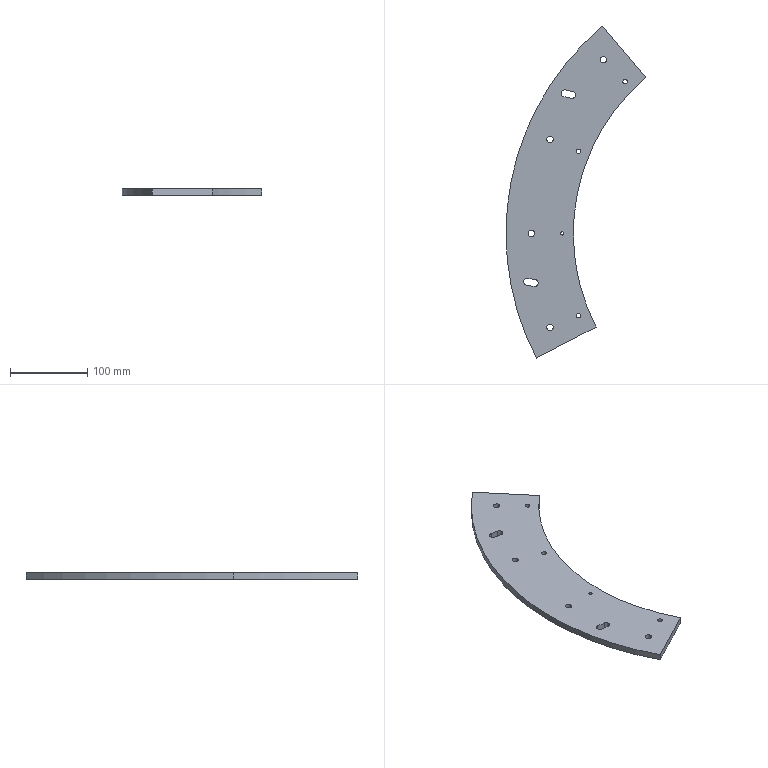Part | 1 solid | 33 faces | box 180.849 x 428.908 x 8 mm | volume 283021 mm3 | cylinder 25 | plane 8 | commonest cylinder face diameters 8.2 x8 6 x6 9 x6 4.174 x2 700 x2 526 x1
STEP:
#1=CARTESIAN_POINT('',(-308.372,-64.185,0.));
#2=VERTEX_POINT('',#1);
#3=CARTESIAN_POINT('',(-311.994,-59.771,0.));
#4=VERTEX_POINT('',#3);
#5=CARTESIAN_POINT('',(-312.872,-64.185,0.));
#6=DIRECTION('',(0.,0.,1.));
#7=DIRECTION('',(1.,0.,0.));
#8=AXIS2_PLACEMENT_3D('',#5,#6,#7);
#9=CIRCLE('',#8,4.5);
#10=EDGE_CURVE('',#2,#4,#9,.T.);
#11=ORIENTED_EDGE('',*,*,#10,.F.);
#12=CARTESIAN_POINT('',(-308.372,-64.185,8.));
#13=VERTEX_POINT('',#12);
#14=CARTESIAN_POINT('',(-308.372,-64.185,-2.));
#15=DIRECTION('',(0.,0.,1.));
#16=VECTOR('',#15,1000.);
#17=LINE('',#14,#16);
#18=EDGE_CURVE('',#2,#13,#17,.T.);
#19=ORIENTED_EDGE('',*,*,#18,.T.);
#20=CARTESIAN_POINT('',(-311.994,-59.771,8.));
#21=VERTEX_POINT('',#20);
#22=CARTESIAN_POINT('',(-312.872,-64.185,8.));
#23=DIRECTION('',(0.,0.,1.));
#24=DIRECTION('',(1.,0.,0.));
#25=AXIS2_PLACEMENT_3D('',#22,#23,#24);
#26=CIRCLE('',#25,4.5);
#27=EDGE_CURVE('',#13,#21,#26,.T.);
#28=ORIENTED_EDGE('',*,*,#27,.T.);
#29=CARTESIAN_POINT('',(-311.994,-59.771,-2.));
#30=DIRECTION('',(0.,0.,1.));
#31=VECTOR('',#30,1000.);
#32=LINE('',#29,#31);
#33=EDGE_CURVE('',#4,#21,#32,.T.);
#34=ORIENTED_EDGE('',*,*,#33,.F.);
#35=EDGE_LOOP('',(#11,#19,#28,#34));
#36=FACE_OUTER_BOUND('',#35,.T.);
#37=CARTESIAN_POINT('',(-312.872,-64.185,-2.));
#38=DIRECTION('',(0.,0.,1.));
#39=DIRECTION('',(1.,0.,0.));
#40=AXIS2_PLACEMENT_3D('',#37,#38,#39);
#41=CYLINDRICAL_SURFACE('',#40,4.5);
#42=ADVANCED_FACE('',(#36),#41,.F.);
#43=CARTESIAN_POINT('',(-259.993,179.03,0.));
#44=VERTEX_POINT('',#43);
#45=CARTESIAN_POINT('',(-263.616,183.444,0.));
#46=VERTEX_POINT('',#45);
#47=CARTESIAN_POINT('',(-264.493,179.03,0.));
#48=DIRECTION('',(0.,0.,1.));
#49=DIRECTION('',(1.,0.,0.));
#50=AXIS2_PLACEMENT_3D('',#47,#48,#49);
#51=CIRCLE('',#50,4.5);
#52=EDGE_CURVE('',#44,#46,#51,.T.);
#53=ORIENTED_EDGE('',*,*,#52,.F.);
#54=CARTESIAN_POINT('',(-259.993,179.03,8.));
#55=VERTEX_POINT('',#54);
#56=CARTESIAN_POINT('',(-259.993,179.03,-2.));
#57=DIRECTION('',(0.,0.,1.));
#58=VECTOR('',#57,1000.);
#59=LINE('',#56,#58);
#60=EDGE_CURVE('',#44,#55,#59,.T.);
#61=ORIENTED_EDGE('',*,*,#60,.T.);
#62=CARTESIAN_POINT('',(-263.616,183.444,8.));
#63=VERTEX_POINT('',#62);
#64=CARTESIAN_POINT('',(-264.493,179.03,8.));
#65=DIRECTION('',(0.,0.,1.));
#66=DIRECTION('',(1.,0.,0.));
#67=AXIS2_PLACEMENT_3D('',#64,#65,#66);
#68=CIRCLE('',#67,4.5);
#69=EDGE_CURVE('',#55,#63,#68,.T.);
#70=ORIENTED_EDGE('',*,*,#69,.T.);
#71=CARTESIAN_POINT('',(-263.616,183.444,-2.));
#72=DIRECTION('',(0.,0.,1.));
#73=VECTOR('',#72,1000.);
#74=LINE('',#71,#73);
#75=EDGE_CURVE('',#46,#63,#74,.T.);
#76=ORIENTED_EDGE('',*,*,#75,.F.);
#77=EDGE_LOOP('',(#53,#61,#70,#76));
#78=FACE_OUTER_BOUND('',#77,.T.);
#79=CARTESIAN_POINT('',(-264.493,179.03,-2.));
#80=DIRECTION('',(0.,0.,1.));
#81=DIRECTION('',(1.,0.,0.));
#82=AXIS2_PLACEMENT_3D('',#79,#80,#81);
#83=CYLINDRICAL_SURFACE('',#82,4.5);
#84=ADVANCED_FACE('',(#78),#83,.F.);
#85=CARTESIAN_POINT('',(-228.457,224.357,0.));
#86=VERTEX_POINT('',#85);
#87=CARTESIAN_POINT('',(-220.257,224.357,0.));
#88=VERTEX_POINT('',#87);
#89=CARTESIAN_POINT('',(-224.357,224.357,0.));
#90=DIRECTION('',(0.,0.,1.));
#91=DIRECTION('',(1.,0.,0.));
#92=AXIS2_PLACEMENT_3D('',#89,#90,#91);
#93=CIRCLE('',#92,4.1);
#94=EDGE_CURVE('',#86,#88,#93,.T.);
#95=ORIENTED_EDGE('',*,*,#94,.F.);
#96=CARTESIAN_POINT('',(-228.457,224.357,8.));
#97=VERTEX_POINT('',#96);
#98=CARTESIAN_POINT('',(-228.457,224.357,-2.));
#99=DIRECTION('',(0.,0.,1.));
#100=VECTOR('',#99,1000.);
#101=LINE('',#98,#100);
#102=EDGE_CURVE('',#86,#97,#101,.T.);
#103=ORIENTED_EDGE('',*,*,#102,.T.);
#104=CARTESIAN_POINT('',(-220.257,224.357,8.));
#105=VERTEX_POINT('',#104);
#106=CARTESIAN_POINT('',(-224.357,224.357,8.));
#107=DIRECTION('',(0.,0.,1.));
#108=DIRECTION('',(1.,0.,0.));
#109=AXIS2_PLACEMENT_3D('',#106,#107,#108);
#110=CIRCLE('',#109,4.1);
#111=EDGE_CURVE('',#97,#105,#110,.T.);
#112=ORIENTED_EDGE('',*,*,#111,.T.);
#113=CARTESIAN_POINT('',(-220.257,224.357,-2.));
#114=DIRECTION('',(0.,0.,1.));
#115=VECTOR('',#114,1000.);
#116=LINE('',#113,#115);
#117=EDGE_CURVE('',#88,#105,#116,.T.);
#118=ORIENTED_EDGE('',*,*,#117,.F.);
#119=EDGE_LOOP('',(#95,#103,#112,#118));
#120=FACE_OUTER_BOUND('',#119,.T.);
#121=CARTESIAN_POINT('',(-224.357,224.357,-2.));
#122=DIRECTION('',(0.,0.,1.));
#123=DIRECTION('',(1.,0.,0.));
#124=AXIS2_PLACEMENT_3D('',#121,#122,#123);
#125=CYLINDRICAL_SURFACE('',#124,4.1);
#126=ADVANCED_FACE('',(#120),#125,.F.);
#127=CARTESIAN_POINT('',(-297.237,121.421,0.));
#128=VERTEX_POINT('',#127);
#129=CARTESIAN_POINT('',(-289.037,121.421,0.));
#130=VERTEX_POINT('',#129);
#131=CARTESIAN_POINT('',(-293.137,121.421,0.));
#132=DIRECTION('',(0.,0.,1.));
#133=DIRECTION('',(1.,0.,0.));
#134=AXIS2_PLACEMENT_3D('',#131,#132,#133);
#135=CIRCLE('',#134,4.1);
#136=EDGE_CURVE('',#128,#130,#135,.T.);
#137=ORIENTED_EDGE('',*,*,#136,.F.);
#138=CARTESIAN_POINT('',(-297.237,121.421,8.));
#139=VERTEX_POINT('',#138);
#140=CARTESIAN_POINT('',(-297.237,121.421,-2.));
#141=DIRECTION('',(0.,0.,1.));
#142=VECTOR('',#141,1000.);
#143=LINE('',#140,#142);
#144=EDGE_CURVE('',#128,#139,#143,.T.);
#145=ORIENTED_EDGE('',*,*,#144,.T.);
#146=CARTESIAN_POINT('',(-289.037,121.421,8.));
#147=VERTEX_POINT('',#146);
#148=CARTESIAN_POINT('',(-293.137,121.421,8.));
#149=DIRECTION('',(0.,0.,1.));
#150=DIRECTION('',(1.,0.,0.));
#151=AXIS2_PLACEMENT_3D('',#148,#149,#150);
#152=CIRCLE('',#151,4.1);
#153=EDGE_CURVE('',#139,#147,#152,.T.);
#154=ORIENTED_EDGE('',*,*,#153,.T.);
#155=CARTESIAN_POINT('',(-289.037,121.421,-2.));
#156=DIRECTION('',(0.,0.,1.));
#157=VECTOR('',#156,1000.);
#158=LINE('',#155,#157);
#159=EDGE_CURVE('',#130,#147,#158,.T.);
#160=ORIENTED_EDGE('',*,*,#159,.F.);
#161=EDGE_LOOP('',(#137,#145,#154,#160));
#162=FACE_OUTER_BOUND('',#161,.T.);
#163=CARTESIAN_POINT('',(-293.137,121.421,-2.));
#164=DIRECTION('',(0.,0.,1.));
#165=DIRECTION('',(1.,0.,0.));
#166=AXIS2_PLACEMENT_3D('',#163,#164,#165);
#167=CYLINDRICAL_SURFACE('',#166,4.1);
#168=ADVANCED_FACE('',(#162),#167,.F.);
#169=CARTESIAN_POINT('',(-321.389,0.,0.));
#170=VERTEX_POINT('',#169);
#171=CARTESIAN_POINT('',(-313.189,0.,0.));
#172=VERTEX_POINT('',#171);
#173=CARTESIAN_POINT('',(-317.289,0.,0.));
#174=DIRECTION('',(0.,0.,1.));
#175=DIRECTION('',(1.,0.,0.));
#176=AXIS2_PLACEMENT_3D('',#173,#174,#175);
#177=CIRCLE('',#176,4.1);
#178=EDGE_CURVE('',#170,#172,#177,.T.);
#179=ORIENTED_EDGE('',*,*,#178,.F.);
#180=CARTESIAN_POINT('',(-321.389,0.,8.));
#181=VERTEX_POINT('',#180);
#182=CARTESIAN_POINT('',(-321.389,0.,-2.));
#183=DIRECTION('',(0.,0.,1.));
#184=VECTOR('',#183,1000.);
#185=LINE('',#182,#184);
#186=EDGE_CURVE('',#170,#181,#185,.T.);
#187=ORIENTED_EDGE('',*,*,#186,.T.);
#188=CARTESIAN_POINT('',(-313.189,0.,8.));
#189=VERTEX_POINT('',#188);
#190=CARTESIAN_POINT('',(-317.289,0.,8.));
#191=DIRECTION('',(0.,0.,1.));
#192=DIRECTION('',(1.,0.,0.));
#193=AXIS2_PLACEMENT_3D('',#190,#191,#192);
#194=CIRCLE('',#193,4.1);
#195=EDGE_CURVE('',#181,#189,#194,.T.);
#196=ORIENTED_EDGE('',*,*,#195,.T.);
#197=CARTESIAN_POINT('',(-313.189,0.,-2.));
#198=DIRECTION('',(0.,0.,1.));
#199=VECTOR('',#198,1000.);
#200=LINE('',#197,#199);
#201=EDGE_CURVE('',#172,#189,#200,.T.);
#202=ORIENTED_EDGE('',*,*,#201,.F.);
#203=EDGE_LOOP('',(#179,#187,#196,#202));
#204=FACE_OUTER_BOUND('',#203,.T.);
#205=CARTESIAN_POINT('',(-317.289,0.,-2.));
#206=DIRECTION('',(0.,0.,1.));
#207=DIRECTION('',(1.,0.,0.));
#208=AXIS2_PLACEMENT_3D('',#205,#206,#207);
#209=CYLINDRICAL_SURFACE('',#208,4.1);
#210=ADVANCED_FACE('',(#204),#209,.F.);
#211=CARTESIAN_POINT('',(-297.237,-121.421,0.));
#212=VERTEX_POINT('',#211);
#213=CARTESIAN_POINT('',(-289.037,-121.421,0.));
#214=VERTEX_POINT('',#213);
#215=CARTESIAN_POINT('',(-293.137,-121.421,0.));
#216=DIRECTION('',(0.,0.,1.));
#217=DIRECTION('',(1.,0.,0.));
#218=AXIS2_PLACEMENT_3D('',#215,#216,#217);
#219=CIRCLE('',#218,4.1);
#220=EDGE_CURVE('',#212,#214,#219,.T.);
#221=ORIENTED_EDGE('',*,*,#220,.F.);
#222=CARTESIAN_POINT('',(-297.237,-121.421,8.));
#223=VERTEX_POINT('',#222);
#224=CARTESIAN_POINT('',(-297.237,-121.421,-2.));
#225=DIRECTION('',(0.,0.,1.));
#226=VECTOR('',#225,1000.);
#227=LINE('',#224,#226);
#228=EDGE_CURVE('',#212,#223,#227,.T.);
#229=ORIENTED_EDGE('',*,*,#228,.T.);
#230=CARTESIAN_POINT('',(-289.037,-121.421,8.));
#231=VERTEX_POINT('',#230);
#232=CARTESIAN_POINT('',(-293.137,-121.421,8.));
#233=DIRECTION('',(0.,0.,1.));
#234=DIRECTION('',(1.,0.,0.));
#235=AXIS2_PLACEMENT_3D('',#232,#233,#234);
#236=CIRCLE('',#235,4.1);
#237=EDGE_CURVE('',#223,#231,#236,.T.);
#238=ORIENTED_EDGE('',*,*,#237,.T.);
#239=CARTESIAN_POINT('',(-289.037,-121.421,-2.));
#240=DIRECTION('',(0.,0.,1.));
#241=VECTOR('',#240,1000.);
#242=LINE('',#239,#241);
#243=EDGE_CURVE('',#214,#231,#242,.T.);
#244=ORIENTED_EDGE('',*,*,#243,.F.);
#245=EDGE_LOOP('',(#221,#229,#238,#244));
#246=FACE_OUTER_BOUND('',#245,.T.);
#247=CARTESIAN_POINT('',(-293.137,-121.421,-2.));
#248=DIRECTION('',(0.,0.,1.));
#249=DIRECTION('',(1.,0.,0.));
#250=AXIS2_PLACEMENT_3D('',#247,#248,#249);
#251=CYLINDRICAL_SURFACE('',#250,4.1);
#252=ADVANCED_FACE('',(#246),#251,.F.);
#253=CARTESIAN_POINT('',(-259.182,-106.114,0.));
#254=VERTEX_POINT('',#253);
#255=CARTESIAN_POINT('',(-253.182,-106.114,0.));
#256=VERTEX_POINT('',#255);
#257=CARTESIAN_POINT('',(-256.182,-106.114,0.));
#258=DIRECTION('',(0.,0.,1.));
#259=DIRECTION('',(1.,0.,0.));
#260=AXIS2_PLACEMENT_3D('',#257,#258,#259);
#261=CIRCLE('',#260,3.);
#262=EDGE_CURVE('',#254,#256,#261,.T.);
#263=ORIENTED_EDGE('',*,*,#262,.F.);
#264=CARTESIAN_POINT('',(-259.182,-106.114,8.));
#265=VERTEX_POINT('',#264);
#266=CARTESIAN_POINT('',(-259.182,-106.114,0.));
#267=DIRECTION('',(0.,0.,1.));
#268=VECTOR('',#267,1000.);
#269=LINE('',#266,#268);
#270=EDGE_CURVE('',#254,#265,#269,.T.);
#271=ORIENTED_EDGE('',*,*,#270,.T.);
#272=CARTESIAN_POINT('',(-253.182,-106.114,8.));
#273=VERTEX_POINT('',#272);
#274=CARTESIAN_POINT('',(-256.182,-106.114,8.));
#275=DIRECTION('',(0.,0.,1.));
#276=DIRECTION('',(1.,0.,0.));
#277=AXIS2_PLACEMENT_3D('',#274,#275,#276);
#278=CIRCLE('',#277,3.);
#279=EDGE_CURVE('',#265,#273,#278,.T.);
#280=ORIENTED_EDGE('',*,*,#279,.T.);
#281=CARTESIAN_POINT('',(-253.182,-106.114,0.));
#282=DIRECTION('',(0.,0.,1.));
#283=VECTOR('',#282,1000.);
#284=LINE('',#281,#283);
#285=EDGE_CURVE('',#256,#273,#284,.T.);
#286=ORIENTED_EDGE('',*,*,#285,.F.);
#287=EDGE_LOOP('',(#263,#271,#280,#286));
#288=FACE_OUTER_BOUND('',#287,.T.);
#289=CARTESIAN_POINT('',(-256.182,-106.114,0.));
#290=DIRECTION('',(0.,0.,1.));
#291=DIRECTION('',(1.,0.,0.));
#292=AXIS2_PLACEMENT_3D('',#289,#290,#291);
#293=CYLINDRICAL_SURFACE('',#292,3.);
#294=ADVANCED_FACE('',(#288),#293,.F.);
#295=CARTESIAN_POINT('',(-279.376,0.,0.));
#296=VERTEX_POINT('',#295);
#297=CARTESIAN_POINT('',(-275.202,0.,0.));
#298=VERTEX_POINT('',#297);
#299=CARTESIAN_POINT('',(-277.289,0.,0.));
#300=DIRECTION('',(0.,0.,1.));
#301=DIRECTION('',(1.,0.,0.));
#302=AXIS2_PLACEMENT_3D('',#299,#300,#301);
#303=CIRCLE('',#302,2.087);
#304=EDGE_CURVE('',#296,#298,#303,.T.);
#305=ORIENTED_EDGE('',*,*,#304,.F.);
#306=CARTESIAN_POINT('',(-279.376,0.,8.));
#307=VERTEX_POINT('',#306);
#308=CARTESIAN_POINT('',(-279.376,0.,0.));
#309=DIRECTION('',(0.,0.,1.));
#310=VECTOR('',#309,1000.);
#311=LINE('',#308,#310);
#312=EDGE_CURVE('',#296,#307,#311,.T.);
#313=ORIENTED_EDGE('',*,*,#312,.T.);
#314=CARTESIAN_POINT('',(-275.202,0.,8.));
#315=VERTEX_POINT('',#314);
#316=CARTESIAN_POINT('',(-277.289,0.,8.));
#317=DIRECTION('',(0.,0.,1.));
#318=DIRECTION('',(1.,0.,0.));
#319=AXIS2_PLACEMENT_3D('',#316,#317,#318);
#320=CIRCLE('',#319,2.087);
#321=EDGE_CURVE('',#307,#315,#320,.T.);
#322=ORIENTED_EDGE('',*,*,#321,.T.);
#323=CARTESIAN_POINT('',(-275.202,0.,0.));
#324=DIRECTION('',(0.,0.,1.));
#325=VECTOR('',#324,1000.);
#326=LINE('',#323,#325);
#327=EDGE_CURVE('',#298,#315,#326,.T.);
#328=ORIENTED_EDGE('',*,*,#327,.F.);
#329=EDGE_LOOP('',(#305,#313,#322,#328));
#330=FACE_OUTER_BOUND('',#329,.T.);
#331=CARTESIAN_POINT('',(-277.289,0.,0.));
#332=DIRECTION('',(0.,0.,1.));
#333=DIRECTION('',(1.,0.,0.));
#334=AXIS2_PLACEMENT_3D('',#331,#332,#333);
#335=CYLINDRICAL_SURFACE('',#334,2.087);
#336=ADVANCED_FACE('',(#330),#335,.F.);
#337=CARTESIAN_POINT('',(-259.182,106.114,0.));
#338=VERTEX_POINT('',#337);
#339=CARTESIAN_POINT('',(-253.182,106.114,0.));
#340=VERTEX_POINT('',#339);
#341=CARTESIAN_POINT('',(-256.182,106.114,0.));
#342=DIRECTION('',(0.,0.,1.));
#343=DIRECTION('',(1.,0.,0.));
#344=AXIS2_PLACEMENT_3D('',#341,#342,#343);
#345=CIRCLE('',#344,3.);
#346=EDGE_CURVE('',#338,#340,#345,.T.);
#347=ORIENTED_EDGE('',*,*,#346,.F.);
#348=CARTESIAN_POINT('',(-259.182,106.114,8.));
#349=VERTEX_POINT('',#348);
#350=CARTESIAN_POINT('',(-259.182,106.114,0.));
#351=DIRECTION('',(0.,0.,1.));
#352=VECTOR('',#351,1000.);
#353=LINE('',#350,#352);
#354=EDGE_CURVE('',#338,#349,#353,.T.);
#355=ORIENTED_EDGE('',*,*,#354,.T.);
#356=CARTESIAN_POINT('',(-253.182,106.114,8.));
#357=VERTEX_POINT('',#356);
#358=CARTESIAN_POINT('',(-256.182,106.114,8.));
#359=DIRECTION('',(0.,0.,1.));
#360=DIRECTION('',(1.,0.,0.));
#361=AXIS2_PLACEMENT_3D('',#358,#359,#360);
#362=CIRCLE('',#361,3.);
#363=EDGE_CURVE('',#349,#357,#362,.T.);
#364=ORIENTED_EDGE('',*,*,#363,.T.);
#365=CARTESIAN_POINT('',(-253.182,106.114,0.));
#366=DIRECTION('',(0.,0.,1.));
#367=VECTOR('',#366,1000.);
#368=LINE('',#365,#367);
#369=EDGE_CURVE('',#340,#357,#368,.T.);
#370=ORIENTED_EDGE('',*,*,#369,.F.);
#371=EDGE_LOOP('',(#347,#355,#364,#370));
#372=FACE_OUTER_BOUND('',#371,.T.);
#373=CARTESIAN_POINT('',(-256.182,106.114,0.));
#374=DIRECTION('',(0.,0.,1.));
#375=DIRECTION('',(1.,0.,0.));
#376=AXIS2_PLACEMENT_3D('',#373,#374,#375);
#377=CYLINDRICAL_SURFACE('',#376,3.);
#378=ADVANCED_FACE('',(#372),#377,.F.);
#379=CARTESIAN_POINT('',(-199.073,196.073,0.));
#380=VERTEX_POINT('',#379);
#381=CARTESIAN_POINT('',(-193.073,196.073,0.));
#382=VERTEX_POINT('',#381);
#383=CARTESIAN_POINT('',(-196.073,196.073,0.));
#384=DIRECTION('',(0.,0.,1.));
#385=DIRECTION('',(1.,0.,0.));
#386=AXIS2_PLACEMENT_3D('',#383,#384,#385);
#387=CIRCLE('',#386,3.);
#388=EDGE_CURVE('',#380,#382,#387,.T.);
#389=ORIENTED_EDGE('',*,*,#388,.F.);
#390=CARTESIAN_POINT('',(-199.073,196.073,8.));
#391=VERTEX_POINT('',#390);
#392=CARTESIAN_POINT('',(-199.073,196.073,0.));
#393=DIRECTION('',(0.,0.,1.));
#394=VECTOR('',#393,1000.);
#395=LINE('',#392,#394);
#396=EDGE_CURVE('',#380,#391,#395,.T.);
#397=ORIENTED_EDGE('',*,*,#396,.T.);
#398=CARTESIAN_POINT('',(-193.073,196.073,8.));
#399=VERTEX_POINT('',#398);
#400=CARTESIAN_POINT('',(-196.073,196.073,8.));
#401=DIRECTION('',(0.,0.,1.));
#402=DIRECTION('',(1.,0.,0.));
#403=AXIS2_PLACEMENT_3D('',#400,#401,#402);
#404=CIRCLE('',#403,3.);
#405=EDGE_CURVE('',#391,#399,#404,.T.);
#406=ORIENTED_EDGE('',*,*,#405,.T.);
#407=CARTESIAN_POINT('',(-193.073,196.073,0.));
#408=DIRECTION('',(0.,0.,1.));
#409=VECTOR('',#408,1000.);
#410=LINE('',#407,#409);
#411=EDGE_CURVE('',#382,#399,#410,.T.);
#412=ORIENTED_EDGE('',*,*,#411,.F.);
#413=EDGE_LOOP('',(#389,#397,#406,#412));
#414=FACE_OUTER_BOUND('',#413,.T.);
#415=CARTESIAN_POINT('',(-196.073,196.073,0.));
#416=DIRECTION('',(0.,0.,1.));
#417=DIRECTION('',(1.,0.,0.));
#418=AXIS2_PLACEMENT_3D('',#415,#416,#417);
#419=CYLINDRICAL_SURFACE('',#418,3.);
#420=ADVANCED_FACE('',(#414),#419,.F.);
#421=CARTESIAN_POINT('',(-350.,0.,8.));
#422=VERTEX_POINT('',#421);
#423=CARTESIAN_POINT('',(-310.823,-160.901,8.));
#424=VERTEX_POINT('',#423);
#425=CARTESIAN_POINT('',(0.,0.,8.));
#426=DIRECTION('',(0.,0.,1.));
#427=DIRECTION('',(1.,0.,0.));
#428=AXIS2_PLACEMENT_3D('',#425,#426,#427);
#429=CIRCLE('',#428,350.);
#430=EDGE_CURVE('',#422,#424,#429,.T.);
#431=ORIENTED_EDGE('',*,*,#430,.F.);
#432=CARTESIAN_POINT('',(-350.,0.,0.));
#433=VERTEX_POINT('',#432);
#434=CARTESIAN_POINT('',(-350.,0.,8.));
#435=DIRECTION('',(0.,0.,-1.));
#436=VECTOR('',#435,1000.);
#437=LINE('',#434,#436);
#438=EDGE_CURVE('',#422,#433,#437,.T.);
#439=ORIENTED_EDGE('',*,*,#438,.T.);
#440=CARTESIAN_POINT('',(-310.823,-160.901,0.));
#441=VERTEX_POINT('',#440);
#442=CARTESIAN_POINT('',(0.,0.,0.));
#443=DIRECTION('',(0.,0.,1.));
#444=DIRECTION('',(1.,0.,0.));
#445=AXIS2_PLACEMENT_3D('',#442,#443,#444);
#446=CIRCLE('',#445,350.);
#447=EDGE_CURVE('',#433,#441,#446,.T.);
#448=ORIENTED_EDGE('',*,*,#447,.T.);
#449=CARTESIAN_POINT('',(-310.823,-160.901,-44.));
#450=DIRECTION('',(0.,0.,1.));
#451=VECTOR('',#450,1000.);
#452=LINE('',#449,#451);
#453=EDGE_CURVE('',#441,#424,#452,.T.);
#454=ORIENTED_EDGE('',*,*,#453,.T.);
#455=EDGE_LOOP('',(#431,#439,#448,#454));
#456=FACE_OUTER_BOUND('',#455,.T.);
#457=CARTESIAN_POINT('',(0.,0.,8.));
#458=DIRECTION('',(0.,0.,-1.));
#459=DIRECTION('',(-1.,0.,0.));
#460=AXIS2_PLACEMENT_3D('',#457,#458,#459);
#461=CYLINDRICAL_SURFACE('',#460,350.);
#462=ADVANCED_FACE('',(#456),#461,.T.);
#463=ORIENTED_EDGE('',*,*,#438,.F.);
#464=CARTESIAN_POINT('',(-225.106,268.006,8.));
#465=VERTEX_POINT('',#464);
#466=CARTESIAN_POINT('',(0.,0.,8.));
#467=DIRECTION('',(0.,0.,1.));
#468=DIRECTION('',(1.,0.,0.));
#469=AXIS2_PLACEMENT_3D('',#466,#467,#468);
#470=CIRCLE('',#469,350.);
#471=EDGE_CURVE('',#465,#422,#470,.T.);
#472=ORIENTED_EDGE('',*,*,#471,.F.);
#473=CARTESIAN_POINT('',(-225.106,268.006,0.));
#474=VERTEX_POINT('',#473);
#475=CARTESIAN_POINT('',(-225.106,268.006,-44.));
#476=DIRECTION('',(0.,0.,1.));
#477=VECTOR('',#476,1000.);
#478=LINE('',#475,#477);
#479=EDGE_CURVE('',#474,#465,#478,.T.);
#480=ORIENTED_EDGE('',*,*,#479,.F.);
#481=CARTESIAN_POINT('',(0.,0.,0.));
#482=DIRECTION('',(0.,0.,1.));
#483=DIRECTION('',(1.,0.,0.));
#484=AXIS2_PLACEMENT_3D('',#481,#482,#483);
#485=CIRCLE('',#484,350.);
#486=EDGE_CURVE('',#474,#433,#485,.T.);
#487=ORIENTED_EDGE('',*,*,#486,.T.);
#488=EDGE_LOOP('',(#463,#472,#480,#487));
#489=FACE_OUTER_BOUND('',#488,.T.);
#490=CARTESIAN_POINT('',(0.,0.,8.));
#491=DIRECTION('',(0.,0.,-1.));
#492=DIRECTION('',(-1.,0.,0.));
#493=AXIS2_PLACEMENT_3D('',#490,#491,#492);
#494=CYLINDRICAL_SURFACE('',#493,350.);
#495=ADVANCED_FACE('',(#489),#494,.T.);
#496=CARTESIAN_POINT('',(-313.75,-68.599,8.));
#497=VERTEX_POINT('',#496);
#498=CARTESIAN_POINT('',(-312.872,-64.185,8.));
#499=DIRECTION('',(0.,0.,1.));
#500=DIRECTION('',(1.,0.,0.));
#501=AXIS2_PLACEMENT_3D('',#498,#499,#500);
#502=CIRCLE('',#501,4.5);
#503=EDGE_CURVE('',#497,#13,#502,.T.);
#504=ORIENTED_EDGE('',*,*,#503,.F.);
#505=CARTESIAN_POINT('',(-323.558,-66.648,8.));
#506=VERTEX_POINT('',#505);
#507=CARTESIAN_POINT('',(-313.75,-68.599,8.));
#508=DIRECTION('',(0.9808,-0.1951,0.));
#509=VECTOR('',#508,1000.);
#510=LINE('',#507,#509);
#511=EDGE_CURVE('',#506,#497,#510,.T.);
#512=ORIENTED_EDGE('',*,*,#511,.F.);
#513=CARTESIAN_POINT('',(-321.802,-57.821,8.));
#514=VERTEX_POINT('',#513);
#515=CARTESIAN_POINT('',(-322.68,-62.234,8.));
#516=DIRECTION('',(0.,0.,1.));
#517=DIRECTION('',(1.,0.,0.));
#518=AXIS2_PLACEMENT_3D('',#515,#516,#517);
#519=CIRCLE('',#518,4.5);
#520=EDGE_CURVE('',#514,#506,#519,.T.);
#521=ORIENTED_EDGE('',*,*,#520,.F.);
#522=CARTESIAN_POINT('',(-311.994,-59.771,8.));
#523=DIRECTION('',(-0.9808,0.1951,0.));
#524=VECTOR('',#523,1000.);
#525=LINE('',#522,#524);
#526=EDGE_CURVE('',#21,#514,#525,.T.);
#527=ORIENTED_EDGE('',*,*,#526,.F.);
#528=ORIENTED_EDGE('',*,*,#27,.F.);
#529=EDGE_LOOP('',(#504,#512,#521,#527,#528));
#530=FACE_BOUND('',#529,.T.);
#531=CARTESIAN_POINT('',(-265.371,174.617,8.));
#532=VERTEX_POINT('',#531);
#533=CARTESIAN_POINT('',(-264.493,179.03,8.));
#534=DIRECTION('',(0.,0.,1.));
#535=DIRECTION('',(1.,0.,0.));
#536=AXIS2_PLACEMENT_3D('',#533,#534,#535);
#537=CIRCLE('',#536,4.5);
#538=EDGE_CURVE('',#532,#55,#537,.T.);
#539=ORIENTED_EDGE('',*,*,#538,.F.);
#540=CARTESIAN_POINT('',(-275.179,176.567,8.));
#541=VERTEX_POINT('',#540);
#542=CARTESIAN_POINT('',(-265.371,174.617,8.));
#543=DIRECTION('',(0.9808,-0.1951,0.));
#544=VECTOR('',#543,1000.);
#545=LINE('',#542,#544);
#546=EDGE_CURVE('',#541,#532,#545,.T.);
#547=ORIENTED_EDGE('',*,*,#546,.F.);
#548=CARTESIAN_POINT('',(-273.423,185.395,8.));
#549=VERTEX_POINT('',#548);
#550=CARTESIAN_POINT('',(-274.301,180.981,8.));
#551=DIRECTION('',(0.,0.,1.));
#552=DIRECTION('',(1.,0.,0.));
#553=AXIS2_PLACEMENT_3D('',#550,#551,#552);
#554=CIRCLE('',#553,4.5);
#555=EDGE_CURVE('',#549,#541,#554,.T.);
#556=ORIENTED_EDGE('',*,*,#555,.F.);
#557=CARTESIAN_POINT('',(-263.616,183.444,8.));
#558=DIRECTION('',(-0.9808,0.1951,0.));
#559=VECTOR('',#558,1000.);
#560=LINE('',#557,#559);
#561=EDGE_CURVE('',#63,#549,#560,.T.);
#562=ORIENTED_EDGE('',*,*,#561,.F.);
#563=ORIENTED_EDGE('',*,*,#69,.F.);
#564=EDGE_LOOP('',(#539,#547,#556,#562,#563));
#565=FACE_BOUND('',#564,.T.);
#566=CARTESIAN_POINT('',(-224.357,224.357,8.));
#567=DIRECTION('',(0.,0.,1.));
#568=DIRECTION('',(1.,0.,0.));
#569=AXIS2_PLACEMENT_3D('',#566,#567,#568);
#570=CIRCLE('',#569,4.1);
#571=EDGE_CURVE('',#105,#97,#570,.T.);
#572=ORIENTED_EDGE('',*,*,#571,.F.);
#573=ORIENTED_EDGE('',*,*,#111,.F.);
#574=EDGE_LOOP('',(#572,#573));
#575=FACE_BOUND('',#574,.T.);
#576=CARTESIAN_POINT('',(-293.137,121.421,8.));
#577=DIRECTION('',(0.,0.,1.));
#578=DIRECTION('',(1.,0.,0.));
#579=AXIS2_PLACEMENT_3D('',#576,#577,#578);
#580=CIRCLE('',#579,4.1);
#581=EDGE_CURVE('',#147,#139,#580,.T.);
#582=ORIENTED_EDGE('',*,*,#581,.F.);
#583=ORIENTED_EDGE('',*,*,#153,.F.);
#584=EDGE_LOOP('',(#582,#583));
#585=FACE_BOUND('',#584,.T.);
#586=CARTESIAN_POINT('',(-317.289,0.,8.));
#587=DIRECTION('',(0.,0.,1.));
#588=DIRECTION('',(1.,0.,0.));
#589=AXIS2_PLACEMENT_3D('',#586,#587,#588);
#590=CIRCLE('',#589,4.1);
#591=EDGE_CURVE('',#189,#181,#590,.T.);
#592=ORIENTED_EDGE('',*,*,#591,.F.);
#593=ORIENTED_EDGE('',*,*,#195,.F.);
#594=EDGE_LOOP('',(#592,#593));
#595=FACE_BOUND('',#594,.T.);
#596=CARTESIAN_POINT('',(-293.137,-121.421,8.));
#597=DIRECTION('',(0.,0.,1.));
#598=DIRECTION('',(1.,0.,0.));
#599=AXIS2_PLACEMENT_3D('',#596,#597,#598);
#600=CIRCLE('',#599,4.1);
#601=EDGE_CURVE('',#231,#223,#600,.T.);
#602=ORIENTED_EDGE('',*,*,#601,.F.);
#603=ORIENTED_EDGE('',*,*,#237,.F.);
#604=EDGE_LOOP('',(#602,#603));
#605=FACE_BOUND('',#604,.T.);
#606=CARTESIAN_POINT('',(-256.182,-106.114,8.));
#607=DIRECTION('',(0.,0.,1.));
#608=DIRECTION('',(1.,0.,0.));
#609=AXIS2_PLACEMENT_3D('',#606,#607,#608);
#610=CIRCLE('',#609,3.);
#611=EDGE_CURVE('',#273,#265,#610,.T.);
#612=ORIENTED_EDGE('',*,*,#611,.F.);
#613=ORIENTED_EDGE('',*,*,#279,.F.);
#614=EDGE_LOOP('',(#612,#613));
#615=FACE_BOUND('',#614,.T.);
#616=CARTESIAN_POINT('',(-277.289,0.,8.));
#617=DIRECTION('',(0.,0.,1.));
#618=DIRECTION('',(1.,0.,0.));
#619=AXIS2_PLACEMENT_3D('',#616,#617,#618);
#620=CIRCLE('',#619,2.087);
#621=EDGE_CURVE('',#315,#307,#620,.T.);
#622=ORIENTED_EDGE('',*,*,#621,.F.);
#623=ORIENTED_EDGE('',*,*,#321,.F.);
#624=EDGE_LOOP('',(#622,#623));
#625=FACE_BOUND('',#624,.T.);
#626=CARTESIAN_POINT('',(-256.182,106.114,8.));
#627=DIRECTION('',(0.,0.,1.));
#628=DIRECTION('',(1.,0.,0.));
#629=AXIS2_PLACEMENT_3D('',#626,#627,#628);
#630=CIRCLE('',#629,3.);
#631=EDGE_CURVE('',#357,#349,#630,.T.);
#632=ORIENTED_EDGE('',*,*,#631,.F.);
#633=ORIENTED_EDGE('',*,*,#363,.F.);
#634=EDGE_LOOP('',(#632,#633));
#635=FACE_BOUND('',#634,.T.);
#636=CARTESIAN_POINT('',(-196.073,196.073,8.));
#637=DIRECTION('',(0.,0.,1.));
#638=DIRECTION('',(1.,0.,0.));
#639=AXIS2_PLACEMENT_3D('',#636,#637,#638);
#640=CIRCLE('',#639,3.);
#641=EDGE_CURVE('',#399,#391,#640,.T.);
#642=ORIENTED_EDGE('',*,*,#641,.F.);
#643=ORIENTED_EDGE('',*,*,#405,.F.);
#644=EDGE_LOOP('',(#642,#643));
#645=FACE_BOUND('',#644,.T.);
#646=CARTESIAN_POINT('',(-169.151,201.388,8.));
#647=VERTEX_POINT('',#646);
#648=CARTESIAN_POINT('',(-233.561,-120.906,8.));
#649=VERTEX_POINT('',#648);
#650=CARTESIAN_POINT('',(0.,0.,8.));
#651=DIRECTION('',(0.,0.,1.));
#652=DIRECTION('',(1.,0.,0.));
#653=AXIS2_PLACEMENT_3D('',#650,#651,#652);
#654=CIRCLE('',#653,263.);
#655=EDGE_CURVE('',#647,#649,#654,.T.);
#656=ORIENTED_EDGE('',*,*,#655,.F.);
#657=CARTESIAN_POINT('',(-169.151,201.388,8.));
#658=DIRECTION('',(0.6432,-0.7657,0.));
#659=VECTOR('',#658,1000.);
#660=LINE('',#657,#659);
#661=EDGE_CURVE('',#465,#647,#660,.T.);
#662=ORIENTED_EDGE('',*,*,#661,.F.);
#663=ORIENTED_EDGE('',*,*,#471,.T.);
#664=ORIENTED_EDGE('',*,*,#430,.T.);
#665=CARTESIAN_POINT('',(-233.561,-120.906,8.));
#666=DIRECTION('',(-0.8881,-0.4597,0.));
#667=VECTOR('',#666,1000.);
#668=LINE('',#665,#667);
#669=EDGE_CURVE('',#649,#424,#668,.T.);
#670=ORIENTED_EDGE('',*,*,#669,.F.);
#671=EDGE_LOOP('',(#656,#662,#663,#664,#670));
#672=FACE_OUTER_BOUND('',#671,.T.);
#673=CARTESIAN_POINT('',(0.,0.,8.));
#674=DIRECTION('',(0.,0.,1.));
#675=DIRECTION('',(1.,0.,0.));
#676=AXIS2_PLACEMENT_3D('',#673,#674,#675);
#677=PLANE('',#676);
#678=ADVANCED_FACE('',(#530,#565,#575,#585,#595,#605,#615,#625,#635,#645,#672),#677,.T.);
#679=CARTESIAN_POINT('',(-224.357,224.357,0.));
#680=DIRECTION('',(0.,0.,1.));
#681=DIRECTION('',(1.,0.,0.));
#682=AXIS2_PLACEMENT_3D('',#679,#680,#681);
#683=CIRCLE('',#682,4.1);
#684=EDGE_CURVE('',#88,#86,#683,.T.);
#685=ORIENTED_EDGE('',*,*,#684,.T.);
#686=ORIENTED_EDGE('',*,*,#94,.T.);
#687=EDGE_LOOP('',(#685,#686));
#688=FACE_BOUND('',#687,.T.);
#689=CARTESIAN_POINT('',(-293.137,121.421,0.));
#690=DIRECTION('',(0.,0.,1.));
#691=DIRECTION('',(1.,0.,0.));
#692=AXIS2_PLACEMENT_3D('',#689,#690,#691);
#693=CIRCLE('',#692,4.1);
#694=EDGE_CURVE('',#130,#128,#693,.T.);
#695=ORIENTED_EDGE('',*,*,#694,.T.);
#696=ORIENTED_EDGE('',*,*,#136,.T.);
#697=EDGE_LOOP('',(#695,#696));
#698=FACE_BOUND('',#697,.T.);
#699=CARTESIAN_POINT('',(-317.289,0.,0.));
#700=DIRECTION('',(0.,0.,1.));
#701=DIRECTION('',(1.,0.,0.));
#702=AXIS2_PLACEMENT_3D('',#699,#700,#701);
#703=CIRCLE('',#702,4.1);
#704=EDGE_CURVE('',#172,#170,#703,.T.);
#705=ORIENTED_EDGE('',*,*,#704,.T.);
#706=ORIENTED_EDGE('',*,*,#178,.T.);
#707=EDGE_LOOP('',(#705,#706));
#708=FACE_BOUND('',#707,.T.);
#709=CARTESIAN_POINT('',(-293.137,-121.421,0.));
#710=DIRECTION('',(0.,0.,1.));
#711=DIRECTION('',(1.,0.,0.));
#712=AXIS2_PLACEMENT_3D('',#709,#710,#711);
#713=CIRCLE('',#712,4.1);
#714=EDGE_CURVE('',#214,#212,#713,.T.);
#715=ORIENTED_EDGE('',*,*,#714,.T.);
#716=ORIENTED_EDGE('',*,*,#220,.T.);
#717=EDGE_LOOP('',(#715,#716));
#718=FACE_BOUND('',#717,.T.);
#719=CARTESIAN_POINT('',(-256.182,-106.114,0.));
#720=DIRECTION('',(0.,0.,1.));
#721=DIRECTION('',(1.,0.,0.));
#722=AXIS2_PLACEMENT_3D('',#719,#720,#721);
#723=CIRCLE('',#722,3.);
#724=EDGE_CURVE('',#256,#254,#723,.T.);
#725=ORIENTED_EDGE('',*,*,#724,.T.);
#726=ORIENTED_EDGE('',*,*,#262,.T.);
#727=EDGE_LOOP('',(#725,#726));
#728=FACE_BOUND('',#727,.T.);
#729=CARTESIAN_POINT('',(-277.289,0.,0.));
#730=DIRECTION('',(0.,0.,1.));
#731=DIRECTION('',(1.,0.,0.));
#732=AXIS2_PLACEMENT_3D('',#729,#730,#731);
#733=CIRCLE('',#732,2.087);
#734=EDGE_CURVE('',#298,#296,#733,.T.);
#735=ORIENTED_EDGE('',*,*,#734,.T.);
#736=ORIENTED_EDGE('',*,*,#304,.T.);
#737=EDGE_LOOP('',(#735,#736));
#738=FACE_BOUND('',#737,.T.);
#739=CARTESIAN_POINT('',(-256.182,106.114,0.));
#740=DIRECTION('',(0.,0.,1.));
#741=DIRECTION('',(1.,0.,0.));
#742=AXIS2_PLACEMENT_3D('',#739,#740,#741);
#743=CIRCLE('',#742,3.);
#744=EDGE_CURVE('',#340,#338,#743,.T.);
#745=ORIENTED_EDGE('',*,*,#744,.T.);
#746=ORIENTED_EDGE('',*,*,#346,.T.);
#747=EDGE_LOOP('',(#745,#746));
#748=FACE_BOUND('',#747,.T.);
#749=CARTESIAN_POINT('',(-196.073,196.073,0.));
#750=DIRECTION('',(0.,0.,1.));
#751=DIRECTION('',(1.,0.,0.));
#752=AXIS2_PLACEMENT_3D('',#749,#750,#751);
#753=CIRCLE('',#752,3.);
#754=EDGE_CURVE('',#382,#380,#753,.T.);
#755=ORIENTED_EDGE('',*,*,#754,.T.);
#756=ORIENTED_EDGE('',*,*,#388,.T.);
#757=EDGE_LOOP('',(#755,#756));
#758=FACE_BOUND('',#757,.T.);
#759=CARTESIAN_POINT('',(-323.558,-66.648,0.));
#760=VERTEX_POINT('',#759);
#761=CARTESIAN_POINT('',(-313.75,-68.599,0.));
#762=VERTEX_POINT('',#761);
#763=CARTESIAN_POINT('',(-25.067,-126.021,0.));
#764=DIRECTION('',(0.9808,-0.1951,0.));
#765=VECTOR('',#764,1000.);
#766=LINE('',#763,#765);
#767=EDGE_CURVE('',#760,#762,#766,.T.);
#768=ORIENTED_EDGE('',*,*,#767,.T.);
#769=CARTESIAN_POINT('',(-312.872,-64.185,0.));
#770=DIRECTION('',(0.,0.,1.));
#771=DIRECTION('',(1.,0.,0.));
#772=AXIS2_PLACEMENT_3D('',#769,#770,#771);
#773=CIRCLE('',#772,4.5);
#774=EDGE_CURVE('',#762,#2,#773,.T.);
#775=ORIENTED_EDGE('',*,*,#774,.T.);
#776=ORIENTED_EDGE('',*,*,#10,.T.);
#777=CARTESIAN_POINT('',(-321.802,-57.821,0.));
#778=VERTEX_POINT('',#777);
#779=CARTESIAN_POINT('',(-23.311,-117.194,0.));
#780=DIRECTION('',(-0.9808,0.1951,0.));
#781=VECTOR('',#780,1000.);
#782=LINE('',#779,#781);
#783=EDGE_CURVE('',#4,#778,#782,.T.);
#784=ORIENTED_EDGE('',*,*,#783,.T.);
#785=CARTESIAN_POINT('',(-322.68,-62.234,0.));
#786=DIRECTION('',(0.,0.,1.));
#787=DIRECTION('',(1.,0.,0.));
#788=AXIS2_PLACEMENT_3D('',#785,#786,#787);
#789=CIRCLE('',#788,4.5);
#790=EDGE_CURVE('',#778,#760,#789,.T.);
#791=ORIENTED_EDGE('',*,*,#790,.T.);
#792=EDGE_LOOP('',(#768,#775,#776,#784,#791));
#793=FACE_BOUND('',#792,.T.);
#794=CARTESIAN_POINT('',(-275.179,176.567,0.));
#795=VERTEX_POINT('',#794);
#796=CARTESIAN_POINT('',(-265.371,174.617,0.));
#797=VERTEX_POINT('',#796);
#798=CARTESIAN_POINT('',(23.311,117.194,0.));
#799=DIRECTION('',(0.9808,-0.1951,0.));
#800=VECTOR('',#799,1000.);
#801=LINE('',#798,#800);
#802=EDGE_CURVE('',#795,#797,#801,.T.);
#803=ORIENTED_EDGE('',*,*,#802,.T.);
#804=CARTESIAN_POINT('',(-264.493,179.03,0.));
#805=DIRECTION('',(0.,0.,1.));
#806=DIRECTION('',(1.,0.,0.));
#807=AXIS2_PLACEMENT_3D('',#804,#805,#806);
#808=CIRCLE('',#807,4.5);
#809=EDGE_CURVE('',#797,#44,#808,.T.);
#810=ORIENTED_EDGE('',*,*,#809,.T.);
#811=ORIENTED_EDGE('',*,*,#52,.T.);
#812=CARTESIAN_POINT('',(-273.423,185.395,0.));
#813=VERTEX_POINT('',#812);
#814=CARTESIAN_POINT('',(25.067,126.021,0.));
#815=DIRECTION('',(-0.9808,0.1951,0.));
#816=VECTOR('',#815,1000.);
#817=LINE('',#814,#816);
#818=EDGE_CURVE('',#46,#813,#817,.T.);
#819=ORIENTED_EDGE('',*,*,#818,.T.);
#820=CARTESIAN_POINT('',(-274.301,180.981,0.));
#821=DIRECTION('',(0.,0.,1.));
#822=DIRECTION('',(1.,0.,0.));
#823=AXIS2_PLACEMENT_3D('',#820,#821,#822);
#824=CIRCLE('',#823,4.5);
#825=EDGE_CURVE('',#813,#795,#824,.T.);
#826=ORIENTED_EDGE('',*,*,#825,.T.);
#827=EDGE_LOOP('',(#803,#810,#811,#819,#826));
#828=FACE_BOUND('',#827,.T.);
#829=CARTESIAN_POINT('',(-169.151,201.388,0.));
#830=VERTEX_POINT('',#829);
#831=CARTESIAN_POINT('',(0.,0.,0.));
#832=DIRECTION('',(0.6432,-0.7657,0.));
#833=VECTOR('',#832,1000.);
#834=LINE('',#831,#833);
#835=EDGE_CURVE('',#474,#830,#834,.T.);
#836=ORIENTED_EDGE('',*,*,#835,.T.);
#837=CARTESIAN_POINT('',(-233.561,-120.906,0.));
#838=VERTEX_POINT('',#837);
#839=CARTESIAN_POINT('',(0.,0.,0.));
#840=DIRECTION('',(0.,0.,1.));
#841=DIRECTION('',(1.,0.,0.));
#842=AXIS2_PLACEMENT_3D('',#839,#840,#841);
#843=CIRCLE('',#842,263.);
#844=EDGE_CURVE('',#830,#838,#843,.T.);
#845=ORIENTED_EDGE('',*,*,#844,.T.);
#846=CARTESIAN_POINT('',(0.,0.,0.));
#847=DIRECTION('',(-0.8881,-0.4597,0.));
#848=VECTOR('',#847,1000.);
#849=LINE('',#846,#848);
#850=EDGE_CURVE('',#838,#441,#849,.T.);
#851=ORIENTED_EDGE('',*,*,#850,.T.);
#852=ORIENTED_EDGE('',*,*,#447,.F.);
#853=ORIENTED_EDGE('',*,*,#486,.F.);
#854=EDGE_LOOP('',(#836,#845,#851,#852,#853));
#855=FACE_OUTER_BOUND('',#854,.T.);
#856=CARTESIAN_POINT('',(0.,0.,0.));
#857=DIRECTION('',(0.,0.,1.));
#858=DIRECTION('',(1.,0.,0.));
#859=AXIS2_PLACEMENT_3D('',#856,#857,#858);
#860=PLANE('',#859);
#861=ADVANCED_FACE('',(#688,#698,#708,#718,#728,#738,#748,#758,#793,#828,#855),#860,.F.);
#862=ORIENTED_EDGE('',*,*,#479,.T.);
#863=ORIENTED_EDGE('',*,*,#661,.T.);
#864=CARTESIAN_POINT('',(-169.151,201.388,-44.));
#865=DIRECTION('',(0.,0.,1.));
#866=VECTOR('',#865,1000.);
#867=LINE('',#864,#866);
#868=EDGE_CURVE('',#830,#647,#867,.T.);
#869=ORIENTED_EDGE('',*,*,#868,.F.);
#870=ORIENTED_EDGE('',*,*,#835,.F.);
#871=EDGE_LOOP('',(#862,#863,#869,#870));
#872=FACE_OUTER_BOUND('',#871,.T.);
#873=CARTESIAN_POINT('',(-169.151,201.388,-44.));
#874=DIRECTION('',(-0.7657,-0.6432,0.));
#875=DIRECTION('',(0.6432,-0.7657,0.));
#876=AXIS2_PLACEMENT_3D('',#873,#874,#875);
#877=PLANE('',#876);
#878=ADVANCED_FACE('',(#872),#877,.F.);
#879=CARTESIAN_POINT('',(-233.561,-120.906,-44.));
#880=DIRECTION('',(0.,0.,1.));
#881=VECTOR('',#880,1000.);
#882=LINE('',#879,#881);
#883=EDGE_CURVE('',#838,#649,#882,.T.);
#884=ORIENTED_EDGE('',*,*,#883,.T.);
#885=ORIENTED_EDGE('',*,*,#669,.T.);
#886=ORIENTED_EDGE('',*,*,#453,.F.);
#887=ORIENTED_EDGE('',*,*,#850,.F.);
#888=EDGE_LOOP('',(#884,#885,#886,#887));
#889=FACE_OUTER_BOUND('',#888,.T.);
#890=CARTESIAN_POINT('',(-233.561,-120.906,-44.));
#891=DIRECTION('',(-0.4597,0.8881,0.));
#892=DIRECTION('',(-0.8881,-0.4597,0.));
#893=AXIS2_PLACEMENT_3D('',#890,#891,#892);
#894=PLANE('',#893);
#895=ADVANCED_FACE('',(#889),#894,.F.);
#896=ORIENTED_EDGE('',*,*,#655,.T.);
#897=ORIENTED_EDGE('',*,*,#883,.F.);
#898=ORIENTED_EDGE('',*,*,#844,.F.);
#899=ORIENTED_EDGE('',*,*,#868,.T.);
#900=EDGE_LOOP('',(#896,#897,#898,#899));
#901=FACE_OUTER_BOUND('',#900,.T.);
#902=CARTESIAN_POINT('',(0.,0.,-44.));
#903=DIRECTION('',(0.,0.,1.));
#904=DIRECTION('',(1.,0.,0.));
#905=AXIS2_PLACEMENT_3D('',#902,#903,#904);
#906=CYLINDRICAL_SURFACE('',#905,263.);
#907=ADVANCED_FACE('',(#901),#906,.F.);
#908=ORIENTED_EDGE('',*,*,#396,.F.);
#909=ORIENTED_EDGE('',*,*,#754,.F.);
#910=ORIENTED_EDGE('',*,*,#411,.T.);
#911=ORIENTED_EDGE('',*,*,#641,.T.);
#912=EDGE_LOOP('',(#908,#909,#910,#911));
#913=FACE_OUTER_BOUND('',#912,.T.);
#914=CARTESIAN_POINT('',(-196.073,196.073,0.));
#915=DIRECTION('',(0.,0.,1.));
#916=DIRECTION('',(1.,0.,0.));
#917=AXIS2_PLACEMENT_3D('',#914,#915,#916);
#918=CYLINDRICAL_SURFACE('',#917,3.);
#919=ADVANCED_FACE('',(#913),#918,.F.);
#920=ORIENTED_EDGE('',*,*,#354,.F.);
#921=ORIENTED_EDGE('',*,*,#744,.F.);
#922=ORIENTED_EDGE('',*,*,#369,.T.);
#923=ORIENTED_EDGE('',*,*,#631,.T.);
#924=EDGE_LOOP('',(#920,#921,#922,#923));
#925=FACE_OUTER_BOUND('',#924,.T.);
#926=CARTESIAN_POINT('',(-256.182,106.114,0.));
#927=DIRECTION('',(0.,0.,1.));
#928=DIRECTION('',(1.,0.,0.));
#929=AXIS2_PLACEMENT_3D('',#926,#927,#928);
#930=CYLINDRICAL_SURFACE('',#929,3.);
#931=ADVANCED_FACE('',(#925),#930,.F.);
#932=ORIENTED_EDGE('',*,*,#312,.F.);
#933=ORIENTED_EDGE('',*,*,#734,.F.);
#934=ORIENTED_EDGE('',*,*,#327,.T.);
#935=ORIENTED_EDGE('',*,*,#621,.T.);
#936=EDGE_LOOP('',(#932,#933,#934,#935));
#937=FACE_OUTER_BOUND('',#936,.T.);
#938=CARTESIAN_POINT('',(-277.289,0.,0.));
#939=DIRECTION('',(0.,0.,1.));
#940=DIRECTION('',(1.,0.,0.));
#941=AXIS2_PLACEMENT_3D('',#938,#939,#940);
#942=CYLINDRICAL_SURFACE('',#941,2.087);
#943=ADVANCED_FACE('',(#937),#942,.F.);
#944=ORIENTED_EDGE('',*,*,#270,.F.);
#945=ORIENTED_EDGE('',*,*,#724,.F.);
#946=ORIENTED_EDGE('',*,*,#285,.T.);
#947=ORIENTED_EDGE('',*,*,#611,.T.);
#948=EDGE_LOOP('',(#944,#945,#946,#947));
#949=FACE_OUTER_BOUND('',#948,.T.);
#950=CARTESIAN_POINT('',(-256.182,-106.114,0.));
#951=DIRECTION('',(0.,0.,1.));
#952=DIRECTION('',(1.,0.,0.));
#953=AXIS2_PLACEMENT_3D('',#950,#951,#952);
#954=CYLINDRICAL_SURFACE('',#953,3.);
#955=ADVANCED_FACE('',(#949),#954,.F.);
#956=ORIENTED_EDGE('',*,*,#228,.F.);
#957=ORIENTED_EDGE('',*,*,#714,.F.);
#958=ORIENTED_EDGE('',*,*,#243,.T.);
#959=ORIENTED_EDGE('',*,*,#601,.T.);
#960=EDGE_LOOP('',(#956,#957,#958,#959));
#961=FACE_OUTER_BOUND('',#960,.T.);
#962=CARTESIAN_POINT('',(-293.137,-121.421,-2.));
#963=DIRECTION('',(0.,0.,1.));
#964=DIRECTION('',(1.,0.,0.));
#965=AXIS2_PLACEMENT_3D('',#962,#963,#964);
#966=CYLINDRICAL_SURFACE('',#965,4.1);
#967=ADVANCED_FACE('',(#961),#966,.F.);
#968=ORIENTED_EDGE('',*,*,#186,.F.);
#969=ORIENTED_EDGE('',*,*,#704,.F.);
#970=ORIENTED_EDGE('',*,*,#201,.T.);
#971=ORIENTED_EDGE('',*,*,#591,.T.);
#972=EDGE_LOOP('',(#968,#969,#970,#971));
#973=FACE_OUTER_BOUND('',#972,.T.);
#974=CARTESIAN_POINT('',(-317.289,0.,-2.));
#975=DIRECTION('',(0.,0.,1.));
#976=DIRECTION('',(1.,0.,0.));
#977=AXIS2_PLACEMENT_3D('',#974,#975,#976);
#978=CYLINDRICAL_SURFACE('',#977,4.1);
#979=ADVANCED_FACE('',(#973),#978,.F.);
#980=ORIENTED_EDGE('',*,*,#144,.F.);
#981=ORIENTED_EDGE('',*,*,#694,.F.);
#982=ORIENTED_EDGE('',*,*,#159,.T.);
#983=ORIENTED_EDGE('',*,*,#581,.T.);
#984=EDGE_LOOP('',(#980,#981,#982,#983));
#985=FACE_OUTER_BOUND('',#984,.T.);
#986=CARTESIAN_POINT('',(-293.137,121.421,-2.));
#987=DIRECTION('',(0.,0.,1.));
#988=DIRECTION('',(1.,0.,0.));
#989=AXIS2_PLACEMENT_3D('',#986,#987,#988);
#990=CYLINDRICAL_SURFACE('',#989,4.1);
#991=ADVANCED_FACE('',(#985),#990,.F.);
#992=ORIENTED_EDGE('',*,*,#102,.F.);
#993=ORIENTED_EDGE('',*,*,#684,.F.);
#994=ORIENTED_EDGE('',*,*,#117,.T.);
#995=ORIENTED_EDGE('',*,*,#571,.T.);
#996=EDGE_LOOP('',(#992,#993,#994,#995));
#997=FACE_OUTER_BOUND('',#996,.T.);
#998=CARTESIAN_POINT('',(-224.357,224.357,-2.));
#999=DIRECTION('',(0.,0.,1.));
#1000=DIRECTION('',(1.,0.,0.));
#1001=AXIS2_PLACEMENT_3D('',#998,#999,#1000);
#1002=CYLINDRICAL_SURFACE('',#1001,4.1);
#1003=ADVANCED_FACE('',(#997),#1002,.F.);
#1004=ORIENTED_EDGE('',*,*,#60,.F.);
#1005=ORIENTED_EDGE('',*,*,#809,.F.);
#1006=CARTESIAN_POINT('',(-265.371,174.617,-2.));
#1007=DIRECTION('',(0.,0.,1.));
#1008=VECTOR('',#1007,1000.);
#1009=LINE('',#1006,#1008);
#1010=EDGE_CURVE('',#797,#532,#1009,.T.);
#1011=ORIENTED_EDGE('',*,*,#1010,.T.);
#1012=ORIENTED_EDGE('',*,*,#538,.T.);
#1013=EDGE_LOOP('',(#1004,#1005,#1011,#1012));
#1014=FACE_OUTER_BOUND('',#1013,.T.);
#1015=CARTESIAN_POINT('',(-264.493,179.03,-2.));
#1016=DIRECTION('',(0.,0.,1.));
#1017=DIRECTION('',(1.,0.,0.));
#1018=AXIS2_PLACEMENT_3D('',#1015,#1016,#1017);
#1019=CYLINDRICAL_SURFACE('',#1018,4.5);
#1020=ADVANCED_FACE('',(#1014),#1019,.F.);
#1021=CARTESIAN_POINT('',(-273.423,185.395,-2.));
#1022=DIRECTION('',(0.,0.,1.));
#1023=VECTOR('',#1022,1000.);
#1024=LINE('',#1021,#1023);
#1025=EDGE_CURVE('',#813,#549,#1024,.T.);
#1026=ORIENTED_EDGE('',*,*,#1025,.T.);
#1027=ORIENTED_EDGE('',*,*,#555,.T.);
#1028=CARTESIAN_POINT('',(-275.179,176.567,-2.));
#1029=DIRECTION('',(0.,0.,1.));
#1030=VECTOR('',#1029,1000.);
#1031=LINE('',#1028,#1030);
#1032=EDGE_CURVE('',#795,#541,#1031,.T.);
#1033=ORIENTED_EDGE('',*,*,#1032,.F.);
#1034=ORIENTED_EDGE('',*,*,#825,.F.);
#1035=EDGE_LOOP('',(#1026,#1027,#1033,#1034));
#1036=FACE_OUTER_BOUND('',#1035,.T.);
#1037=CARTESIAN_POINT('',(-274.301,180.981,-2.));
#1038=DIRECTION('',(0.,0.,1.));
#1039=DIRECTION('',(1.,0.,0.));
#1040=AXIS2_PLACEMENT_3D('',#1037,#1038,#1039);
#1041=CYLINDRICAL_SURFACE('',#1040,4.5);
#1042=ADVANCED_FACE('',(#1036),#1041,.F.);
#1043=ORIENTED_EDGE('',*,*,#1032,.T.);
#1044=ORIENTED_EDGE('',*,*,#546,.T.);
#1045=ORIENTED_EDGE('',*,*,#1010,.F.);
#1046=ORIENTED_EDGE('',*,*,#802,.F.);
#1047=EDGE_LOOP('',(#1043,#1044,#1045,#1046));
#1048=FACE_OUTER_BOUND('',#1047,.T.);
#1049=CARTESIAN_POINT('',(-265.371,174.617,-2.));
#1050=DIRECTION('',(-0.1951,-0.9808,0.));
#1051=DIRECTION('',(0.9808,-0.1951,0.));
#1052=AXIS2_PLACEMENT_3D('',#1049,#1050,#1051);
#1053=PLANE('',#1052);
#1054=ADVANCED_FACE('',(#1048),#1053,.F.);
#1055=ORIENTED_EDGE('',*,*,#75,.T.);
#1056=ORIENTED_EDGE('',*,*,#561,.T.);
#1057=ORIENTED_EDGE('',*,*,#1025,.F.);
#1058=ORIENTED_EDGE('',*,*,#818,.F.);
#1059=EDGE_LOOP('',(#1055,#1056,#1057,#1058));
#1060=FACE_OUTER_BOUND('',#1059,.T.);
#1061=CARTESIAN_POINT('',(-263.616,183.444,-2.));
#1062=DIRECTION('',(0.1951,0.9808,0.));
#1063=DIRECTION('',(-0.9808,0.1951,0.));
#1064=AXIS2_PLACEMENT_3D('',#1061,#1062,#1063);
#1065=PLANE('',#1064);
#1066=ADVANCED_FACE('',(#1060),#1065,.F.);
#1067=ORIENTED_EDGE('',*,*,#18,.F.);
#1068=ORIENTED_EDGE('',*,*,#774,.F.);
#1069=CARTESIAN_POINT('',(-313.75,-68.599,-2.));
#1070=DIRECTION('',(0.,0.,1.));
#1071=VECTOR('',#1070,1000.);
#1072=LINE('',#1069,#1071);
#1073=EDGE_CURVE('',#762,#497,#1072,.T.);
#1074=ORIENTED_EDGE('',*,*,#1073,.T.);
#1075=ORIENTED_EDGE('',*,*,#503,.T.);
#1076=EDGE_LOOP('',(#1067,#1068,#1074,#1075));
#1077=FACE_OUTER_BOUND('',#1076,.T.);
#1078=CARTESIAN_POINT('',(-312.872,-64.185,-2.));
#1079=DIRECTION('',(0.,0.,1.));
#1080=DIRECTION('',(1.,0.,0.));
#1081=AXIS2_PLACEMENT_3D('',#1078,#1079,#1080);
#1082=CYLINDRICAL_SURFACE('',#1081,4.5);
#1083=ADVANCED_FACE('',(#1077),#1082,.F.);
#1084=CARTESIAN_POINT('',(-321.802,-57.821,-2.));
#1085=DIRECTION('',(0.,0.,1.));
#1086=VECTOR('',#1085,1000.);
#1087=LINE('',#1084,#1086);
#1088=EDGE_CURVE('',#778,#514,#1087,.T.);
#1089=ORIENTED_EDGE('',*,*,#1088,.T.);
#1090=ORIENTED_EDGE('',*,*,#520,.T.);
#1091=CARTESIAN_POINT('',(-323.558,-66.648,-2.));
#1092=DIRECTION('',(0.,0.,1.));
#1093=VECTOR('',#1092,1000.);
#1094=LINE('',#1091,#1093);
#1095=EDGE_CURVE('',#760,#506,#1094,.T.);
#1096=ORIENTED_EDGE('',*,*,#1095,.F.);
#1097=ORIENTED_EDGE('',*,*,#790,.F.);
#1098=EDGE_LOOP('',(#1089,#1090,#1096,#1097));
#1099=FACE_OUTER_BOUND('',#1098,.T.);
#1100=CARTESIAN_POINT('',(-322.68,-62.234,-2.));
#1101=DIRECTION('',(0.,0.,1.));
#1102=DIRECTION('',(1.,0.,0.));
#1103=AXIS2_PLACEMENT_3D('',#1100,#1101,#1102);
#1104=CYLINDRICAL_SURFACE('',#1103,4.5);
#1105=ADVANCED_FACE('',(#1099),#1104,.F.);
#1106=ORIENTED_EDGE('',*,*,#1095,.T.);
#1107=ORIENTED_EDGE('',*,*,#511,.T.);
#1108=ORIENTED_EDGE('',*,*,#1073,.F.);
#1109=ORIENTED_EDGE('',*,*,#767,.F.);
#1110=EDGE_LOOP('',(#1106,#1107,#1108,#1109));
#1111=FACE_OUTER_BOUND('',#1110,.T.);
#1112=CARTESIAN_POINT('',(-313.75,-68.599,-2.));
#1113=DIRECTION('',(-0.1951,-0.9808,0.));
#1114=DIRECTION('',(0.9808,-0.1951,0.));
#1115=AXIS2_PLACEMENT_3D('',#1112,#1113,#1114);
#1116=PLANE('',#1115);
#1117=ADVANCED_FACE('',(#1111),#1116,.F.);
#1118=ORIENTED_EDGE('',*,*,#33,.T.);
#1119=ORIENTED_EDGE('',*,*,#526,.T.);
#1120=ORIENTED_EDGE('',*,*,#1088,.F.);
#1121=ORIENTED_EDGE('',*,*,#783,.F.);
#1122=EDGE_LOOP('',(#1118,#1119,#1120,#1121));
#1123=FACE_OUTER_BOUND('',#1122,.T.);
#1124=CARTESIAN_POINT('',(-311.994,-59.771,-2.));
#1125=DIRECTION('',(0.1951,0.9808,0.));
#1126=DIRECTION('',(-0.9808,0.1951,0.));
#1127=AXIS2_PLACEMENT_3D('',#1124,#1125,#1126);
#1128=PLANE('',#1127);
#1129=ADVANCED_FACE('',(#1123),#1128,.F.);
#1130=CLOSED_SHELL('',(#42,#84,#126,#168,#210,#252,#294,#336,#378,#420,#462,#495,#678,#861,#878,#895,#907,#919,#931,#943,#955,#967,#979,#991,#1003,#1020,#1042,#1054,#1066,#1083,#1105,#1117,#1129));
#1131=MANIFOLD_SOLID_BREP('',#1130);
#1132=CARTESIAN_POINT('',(0.,0.,0.));
#1133=DIRECTION('',(0.,0.,1.));
#1134=DIRECTION('',(1.,0.,0.));
#1135=AXIS2_PLACEMENT_3D('',#1132,#1133,#1134);
#1136=(LENGTH_UNIT()NAMED_UNIT(*)SI_UNIT(.MILLI.,.METRE.));
#1137=UNCERTAINTY_MEASURE_WITH_UNIT(LENGTH_MEASURE(0.00001),#1136,'','');
#1138=(NAMED_UNIT(*)PLANE_ANGLE_UNIT()SI_UNIT($,.RADIAN.));
#1139=(NAMED_UNIT(*)SI_UNIT($,.STERADIAN.)SOLID_ANGLE_UNIT());
#1140=(GEOMETRIC_REPRESENTATION_CONTEXT(3)GLOBAL_UNCERTAINTY_ASSIGNED_CONTEXT((#1137))GLOBAL_UNIT_ASSIGNED_CONTEXT((#1136,#1138,#1139))REPRESENTATION_CONTEXT('',''));
#1141=ADVANCED_BREP_SHAPE_REPRESENTATION('',(#1131,#1135),#1140);